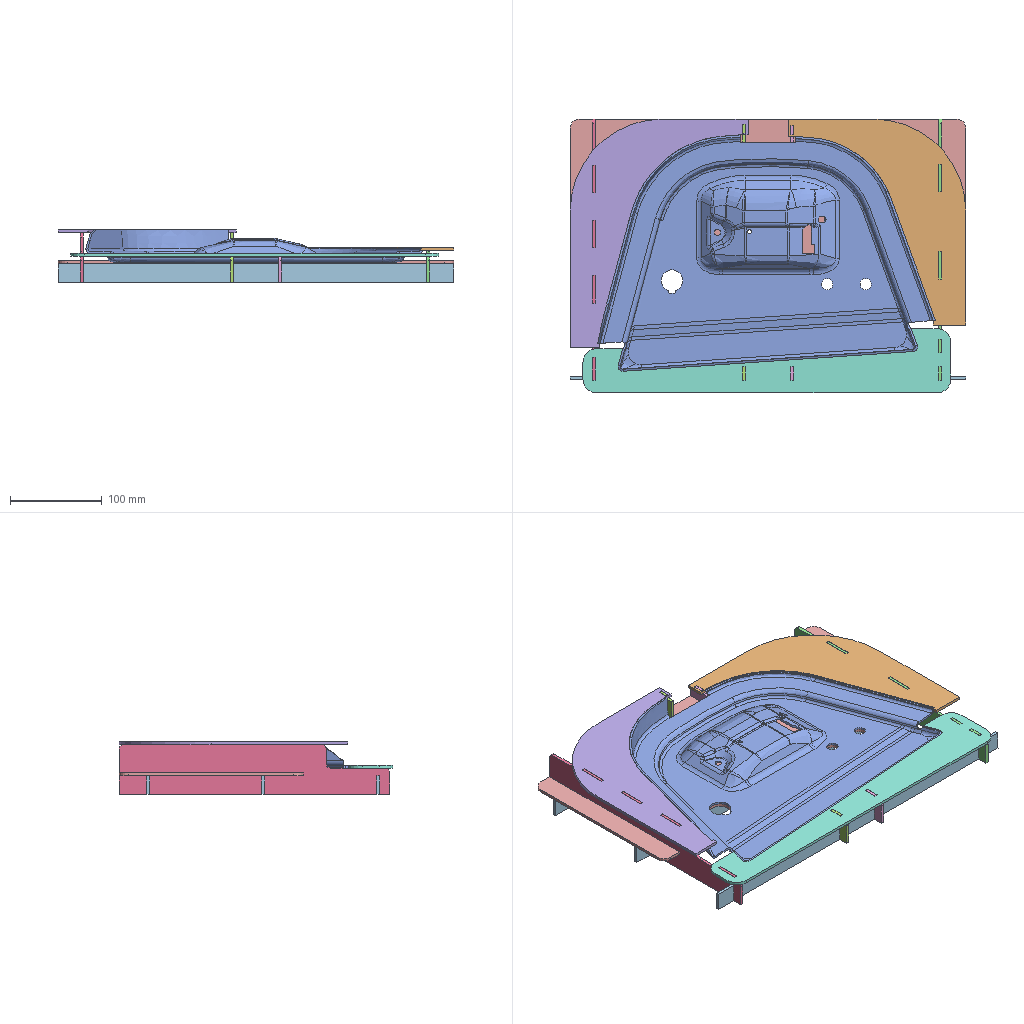Assembly | SolidWorks | 10 different items | 12 placed | box 430 x 298 x 57 mm
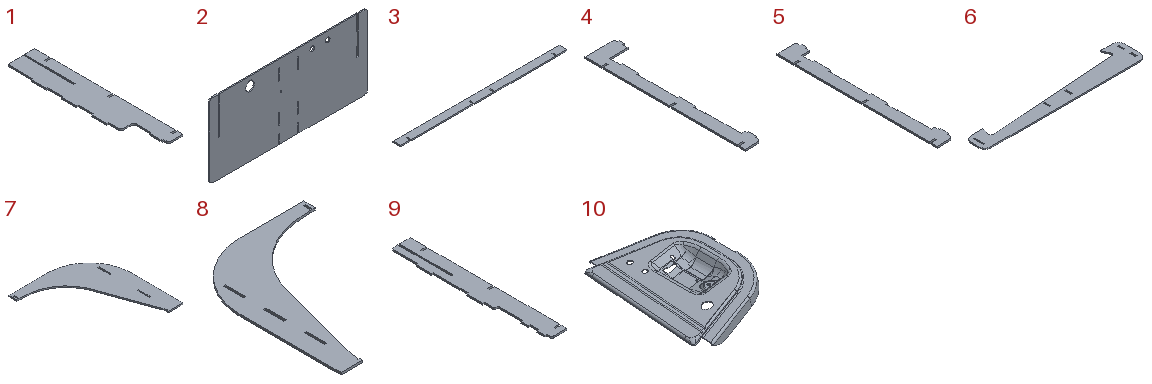Parts list (item | quantity | size | volume | features):
1 | x1 | 57 x 294.081 x 3.2 mm | 44908 mm3 | features FlatPattern 1, SMBaseFlange 1, SheetMetal 1
2 | x1 | 430 x 3.2 x 200 mm | 268842 mm3 | features FlatPattern 1, SMBaseFlange 1, SheetMetal 1
3 | x3 | 430 x 20 x 3.2 mm | 27110 mm3 | features FlatPattern 1, SMBaseFlange 1, SheetMetal 1
4 | x1 | 57 x 294.081 x 3.2 mm | 23149 mm3 | features FlatPattern 1, SMBaseFlange 1, SheetMetal 1
5 | x1 | 38 x 294.081 x 3.2 mm | 21708 mm3 | features FlatPattern 1, SMBaseFlange 1, SheetMetal 1
6 | x1 | 400 x 70 x 3.2 mm | 48547 mm3 | features FlatPattern 1, SMBaseFlange 1, SheetMetal 1
7 | x1 | 192.85 x 223.811 x 3.2 mm | 52018 mm3 | features FlatPattern 1, SMBaseFlange 1, SheetMetal 1
8 | x1 | 193.405 x 248.788 x 3.2 mm | 50560 mm3 | features FlatPattern 1, SMBaseFlange 1, SheetMetal 1
9 | x1 | 38 x 294.081 x 3.2 mm | 30340 mm3 | features FlatPattern 1, SMBaseFlange 1, SheetMetal 1
10 | x1 | 258.18 x 367.01 x 57.896 mm | 192085 mm3 | features BaseBody 1
Mates (type | each side: item.copy, entity, surface, feature):
Coincident | 2.1 face plane Base-Flange1 | 10.1 face plane Input1
DistanceDim | 10.1 edge | 2.1 face plane Base-Flange1
Coincident | 10.1 edge | assembly plane
InPlace | 4.1 plane | assembly plane
Coincident | 4.1 face plane Base-Flange1 | 5.1 face plane Base-Flange1
DistanceDim | 4.1 face plane Base-Flange1 | 5.1 face plane Base-Flange1
InPlace | 4.1 face plane Base-Flange1 | 6.1 plane
InPlace | 7.1 plane | assembly plane
InPlace | 8.1 plane | assembly plane
InPlace | 9.1 plane | assembly plane
InPlace | 3.1 plane | assembly plane